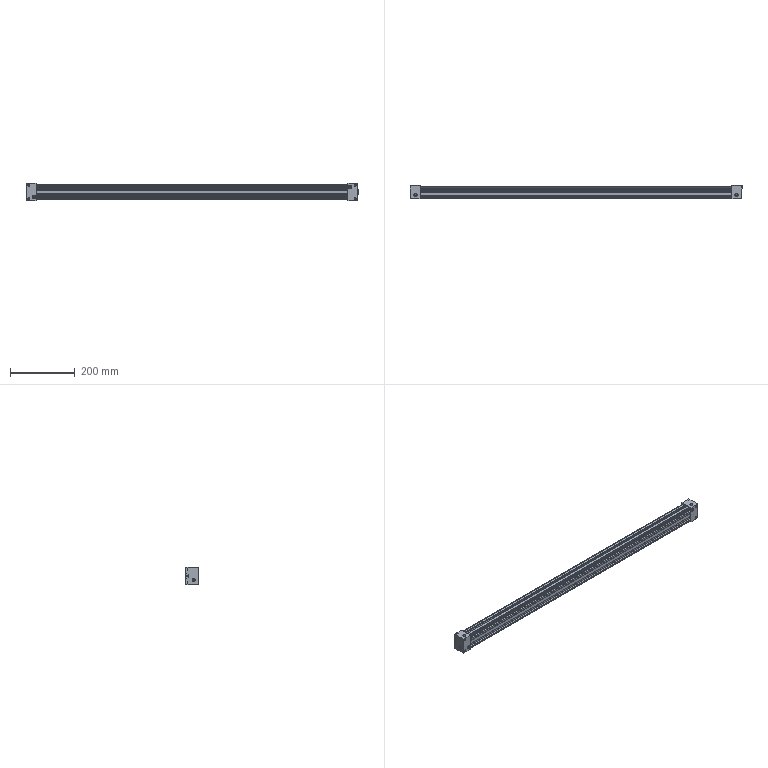Part | SolidWorks | features BaseBody 1 | 1 solid | 299 faces | box 1022 x 40.5 x 53 mm | volume 1560692 mm3 | plane 183 | cylinder 88 | cone 20 | spline 8 | commonest cylinder face diameters 2 x21 5.5 x8 5.6 x8 9 x8 9.728 x8 6 x6